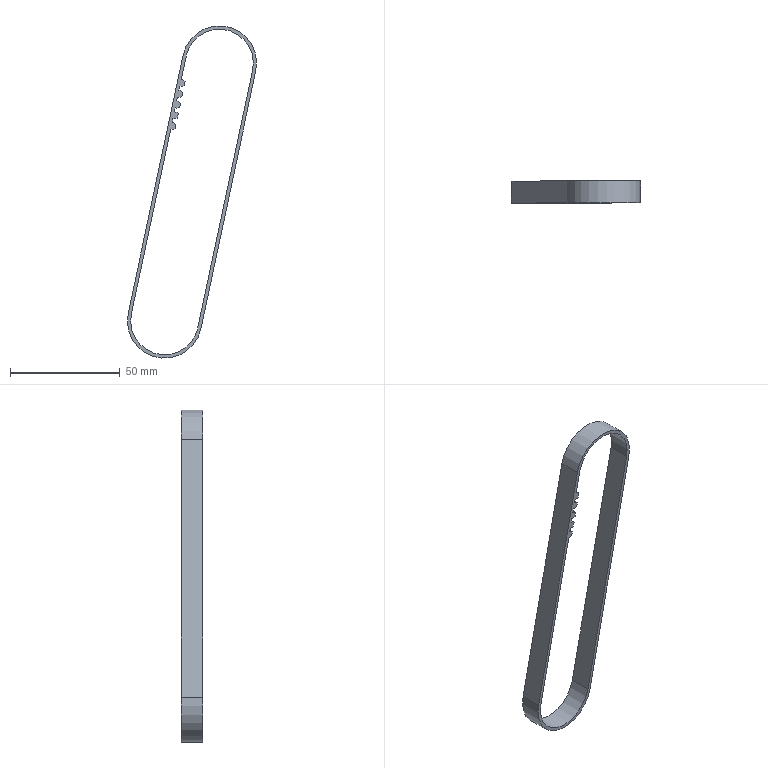Part | STEP file | ROTATION MC_NEW VER-0610_583 | 1 solid | 30 faces | box 58.82 x 10 x 151.249 mm | volume 5398 mm3 | plane 16 | cylinder 14 | commonest cylinder face diameters 6.5 x10 30.871 x2 33.871 x2
STEP:
#1=CARTESIAN_POINT('',(-250.868,696.008,-98.41));
#2=VERTEX_POINT('',#1);
#3=CARTESIAN_POINT('',(-249.129,696.008,-99.414));
#4=VERTEX_POINT('',#3);
#5=CARTESIAN_POINT('',(-251.544,696.008,-101.589));
#6=DIRECTION('',(0.,1.,0.));
#7=DIRECTION('',(-0.2079,0.,-0.9781));
#8=AXIS2_PLACEMENT_3D('',#5,#6,#7);
#9=CIRCLE('',#8,3.25);
#10=EDGE_CURVE('',#2,#4,#9,.T.);
#11=ORIENTED_EDGE('',*,*,#10,.T.);
#12=CARTESIAN_POINT('',(-249.129,706.008,-99.414));
#13=VERTEX_POINT('',#12);
#14=CARTESIAN_POINT('',(-249.129,706.008,-99.414));
#15=DIRECTION('',(0.,-1.,0.));
#16=VECTOR('',#15,10.);
#17=LINE('',#14,#16);
#18=EDGE_CURVE('',#13,#4,#17,.T.);
#19=ORIENTED_EDGE('',*,*,#18,.F.);
#20=CARTESIAN_POINT('',(-250.868,706.008,-98.41));
#21=VERTEX_POINT('',#20);
#22=CARTESIAN_POINT('',(-251.544,706.008,-101.589));
#23=DIRECTION('',(0.,1.,0.));
#24=DIRECTION('',(-0.2079,0.,-0.9781));
#25=AXIS2_PLACEMENT_3D('',#22,#23,#24);
#26=CIRCLE('',#25,3.25);
#27=EDGE_CURVE('',#21,#13,#26,.T.);
#28=ORIENTED_EDGE('',*,*,#27,.F.);
#29=CARTESIAN_POINT('',(-250.868,706.008,-98.41));
#30=DIRECTION('',(0.,-1.,0.));
#31=VECTOR('',#30,10.);
#32=LINE('',#29,#31);
#33=EDGE_CURVE('',#21,#2,#32,.T.);
#34=ORIENTED_EDGE('',*,*,#33,.T.);
#35=EDGE_LOOP('',(#11,#19,#28,#34));
#36=FACE_OUTER_BOUND('',#35,.T.);
#37=CARTESIAN_POINT('',(-251.544,706.008,-101.589));
#38=DIRECTION('',(0.,1.,0.));
#39=DIRECTION('',(-0.2079,0.,-0.9781));
#40=AXIS2_PLACEMENT_3D('',#37,#38,#39);
#41=CYLINDRICAL_SURFACE('',#40,3.25);
#42=ADVANCED_FACE('',(#36),#41,.T.);
#43=CARTESIAN_POINT('',(-249.547,696.008,-101.379));
#44=VERTEX_POINT('',#43);
#45=CARTESIAN_POINT('',(-249.129,696.008,-99.414));
#46=DIRECTION('',(-0.2079,0.,-0.9781));
#47=VECTOR('',#46,2.009);
#48=LINE('',#45,#47);
#49=EDGE_CURVE('',#4,#44,#48,.T.);
#50=ORIENTED_EDGE('',*,*,#49,.T.);
#51=CARTESIAN_POINT('',(-249.547,706.008,-101.379));
#52=VERTEX_POINT('',#51);
#53=CARTESIAN_POINT('',(-249.547,706.008,-101.379));
#54=DIRECTION('',(0.,-1.,0.));
#55=VECTOR('',#54,10.);
#56=LINE('',#53,#55);
#57=EDGE_CURVE('',#52,#44,#56,.T.);
#58=ORIENTED_EDGE('',*,*,#57,.F.);
#59=CARTESIAN_POINT('',(-249.129,706.008,-99.414));
#60=DIRECTION('',(-0.2079,0.,-0.9781));
#61=VECTOR('',#60,2.009);
#62=LINE('',#59,#61);
#63=EDGE_CURVE('',#13,#52,#62,.T.);
#64=ORIENTED_EDGE('',*,*,#63,.F.);
#65=ORIENTED_EDGE('',*,*,#18,.T.);
#66=EDGE_LOOP('',(#50,#58,#64,#65));
#67=FACE_OUTER_BOUND('',#66,.T.);
#68=CARTESIAN_POINT('',(-249.129,706.008,-99.414));
#69=DIRECTION('',(-0.9781,0.,0.2079));
#70=DIRECTION('',(0.2079,0.,0.9781));
#71=AXIS2_PLACEMENT_3D('',#68,#69,#70);
#72=PLANE('',#71);
#73=ADVANCED_FACE('',(#67),#72,.F.);
#74=CARTESIAN_POINT('',(-251.544,696.008,-101.589));
#75=VERTEX_POINT('',#74);
#76=CARTESIAN_POINT('',(-250.868,696.008,-98.41));
#77=DIRECTION('',(0.,1.,0.));
#78=DIRECTION('',(-0.2079,0.,-0.9781));
#79=AXIS2_PLACEMENT_3D('',#76,#77,#78);
#80=CIRCLE('',#79,3.25);
#81=EDGE_CURVE('',#44,#75,#80,.T.);
#82=ORIENTED_EDGE('',*,*,#81,.T.);
#83=CARTESIAN_POINT('',(-251.544,706.008,-101.589));
#84=VERTEX_POINT('',#83);
#85=CARTESIAN_POINT('',(-251.544,706.008,-101.589));
#86=DIRECTION('',(0.,-1.,0.));
#87=VECTOR('',#86,10.);
#88=LINE('',#85,#87);
#89=EDGE_CURVE('',#84,#75,#88,.T.);
#90=ORIENTED_EDGE('',*,*,#89,.F.);
#91=CARTESIAN_POINT('',(-250.868,706.008,-98.41));
#92=DIRECTION('',(0.,1.,0.));
#93=DIRECTION('',(-0.2079,0.,-0.9781));
#94=AXIS2_PLACEMENT_3D('',#91,#92,#93);
#95=CIRCLE('',#94,3.25);
#96=EDGE_CURVE('',#52,#84,#95,.T.);
#97=ORIENTED_EDGE('',*,*,#96,.F.);
#98=ORIENTED_EDGE('',*,*,#57,.T.);
#99=EDGE_LOOP('',(#82,#90,#97,#98));
#100=FACE_OUTER_BOUND('',#99,.T.);
#101=CARTESIAN_POINT('',(-250.868,706.008,-98.41));
#102=DIRECTION('',(0.,1.,0.));
#103=DIRECTION('',(-0.2079,0.,-0.9781));
#104=AXIS2_PLACEMENT_3D('',#101,#102,#103);
#105=CYLINDRICAL_SURFACE('',#104,3.25);
#106=ADVANCED_FACE('',(#100),#105,.T.);
#107=CARTESIAN_POINT('',(-251.908,696.008,-103.301));
#108=VERTEX_POINT('',#107);
#109=CARTESIAN_POINT('',(-251.544,696.008,-101.589));
#110=DIRECTION('',(-0.2079,0.,-0.9781));
#111=VECTOR('',#110,1.75);
#112=LINE('',#109,#111);
#113=EDGE_CURVE('',#75,#108,#112,.T.);
#114=ORIENTED_EDGE('',*,*,#113,.T.);
#115=CARTESIAN_POINT('',(-251.908,706.008,-103.301));
#116=VERTEX_POINT('',#115);
#117=CARTESIAN_POINT('',(-251.908,706.008,-103.301));
#118=DIRECTION('',(0.,-1.,0.));
#119=VECTOR('',#118,10.);
#120=LINE('',#117,#119);
#121=EDGE_CURVE('',#116,#108,#120,.T.);
#122=ORIENTED_EDGE('',*,*,#121,.F.);
#123=CARTESIAN_POINT('',(-251.544,706.008,-101.589));
#124=DIRECTION('',(-0.2079,0.,-0.9781));
#125=VECTOR('',#124,1.75);
#126=LINE('',#123,#125);
#127=EDGE_CURVE('',#84,#116,#126,.T.);
#128=ORIENTED_EDGE('',*,*,#127,.F.);
#129=ORIENTED_EDGE('',*,*,#89,.T.);
#130=EDGE_LOOP('',(#114,#122,#128,#129));
#131=FACE_OUTER_BOUND('',#130,.T.);
#132=CARTESIAN_POINT('',(-251.544,706.008,-101.589));
#133=DIRECTION('',(-0.9781,0.,0.2079));
#134=DIRECTION('',(0.2079,0.,0.9781));
#135=AXIS2_PLACEMENT_3D('',#132,#133,#134);
#136=PLANE('',#135);
#137=ADVANCED_FACE('',(#131),#136,.F.);
#138=CARTESIAN_POINT('',(-250.168,696.008,-104.305));
#139=VERTEX_POINT('',#138);
#140=CARTESIAN_POINT('',(-252.583,696.008,-106.48));
#141=DIRECTION('',(0.,1.,0.));
#142=DIRECTION('',(-0.2079,0.,-0.9781));
#143=AXIS2_PLACEMENT_3D('',#140,#141,#142);
#144=CIRCLE('',#143,3.25);
#145=EDGE_CURVE('',#108,#139,#144,.T.);
#146=ORIENTED_EDGE('',*,*,#145,.T.);
#147=CARTESIAN_POINT('',(-250.168,706.008,-104.305));
#148=VERTEX_POINT('',#147);
#149=CARTESIAN_POINT('',(-250.168,706.008,-104.305));
#150=DIRECTION('',(0.,-1.,0.));
#151=VECTOR('',#150,10.);
#152=LINE('',#149,#151);
#153=EDGE_CURVE('',#148,#139,#152,.T.);
#154=ORIENTED_EDGE('',*,*,#153,.F.);
#155=CARTESIAN_POINT('',(-252.583,706.008,-106.48));
#156=DIRECTION('',(0.,1.,0.));
#157=DIRECTION('',(-0.2079,0.,-0.9781));
#158=AXIS2_PLACEMENT_3D('',#155,#156,#157);
#159=CIRCLE('',#158,3.25);
#160=EDGE_CURVE('',#116,#148,#159,.T.);
#161=ORIENTED_EDGE('',*,*,#160,.F.);
#162=ORIENTED_EDGE('',*,*,#121,.T.);
#163=EDGE_LOOP('',(#146,#154,#161,#162));
#164=FACE_OUTER_BOUND('',#163,.T.);
#165=CARTESIAN_POINT('',(-252.583,706.008,-106.48));
#166=DIRECTION('',(0.,1.,0.));
#167=DIRECTION('',(-0.2079,0.,-0.9781));
#168=AXIS2_PLACEMENT_3D('',#165,#166,#167);
#169=CYLINDRICAL_SURFACE('',#168,3.25);
#170=ADVANCED_FACE('',(#164),#169,.T.);
#171=CARTESIAN_POINT('',(-250.586,696.008,-106.27));
#172=VERTEX_POINT('',#171);
#173=CARTESIAN_POINT('',(-250.168,696.008,-104.305));
#174=DIRECTION('',(-0.2079,0.,-0.9781));
#175=VECTOR('',#174,2.009);
#176=LINE('',#173,#175);
#177=EDGE_CURVE('',#139,#172,#176,.T.);
#178=ORIENTED_EDGE('',*,*,#177,.T.);
#179=CARTESIAN_POINT('',(-250.586,706.008,-106.27));
#180=VERTEX_POINT('',#179);
#181=CARTESIAN_POINT('',(-250.586,706.008,-106.27));
#182=DIRECTION('',(0.,-1.,0.));
#183=VECTOR('',#182,10.);
#184=LINE('',#181,#183);
#185=EDGE_CURVE('',#180,#172,#184,.T.);
#186=ORIENTED_EDGE('',*,*,#185,.F.);
#187=CARTESIAN_POINT('',(-250.168,706.008,-104.305));
#188=DIRECTION('',(-0.2079,0.,-0.9781));
#189=VECTOR('',#188,2.009);
#190=LINE('',#187,#189);
#191=EDGE_CURVE('',#148,#180,#190,.T.);
#192=ORIENTED_EDGE('',*,*,#191,.F.);
#193=ORIENTED_EDGE('',*,*,#153,.T.);
#194=EDGE_LOOP('',(#178,#186,#192,#193));
#195=FACE_OUTER_BOUND('',#194,.T.);
#196=CARTESIAN_POINT('',(-250.168,706.008,-104.305));
#197=DIRECTION('',(-0.9781,0.,0.2079));
#198=DIRECTION('',(0.2079,0.,0.9781));
#199=AXIS2_PLACEMENT_3D('',#196,#197,#198);
#200=PLANE('',#199);
#201=ADVANCED_FACE('',(#195),#200,.F.);
#202=CARTESIAN_POINT('',(-252.583,696.008,-106.48));
#203=VERTEX_POINT('',#202);
#204=CARTESIAN_POINT('',(-251.908,696.008,-103.301));
#205=DIRECTION('',(0.,1.,0.));
#206=DIRECTION('',(-0.2079,0.,-0.9781));
#207=AXIS2_PLACEMENT_3D('',#204,#205,#206);
#208=CIRCLE('',#207,3.25);
#209=EDGE_CURVE('',#172,#203,#208,.T.);
#210=ORIENTED_EDGE('',*,*,#209,.T.);
#211=CARTESIAN_POINT('',(-252.583,706.008,-106.48));
#212=VERTEX_POINT('',#211);
#213=CARTESIAN_POINT('',(-252.583,706.008,-106.48));
#214=DIRECTION('',(0.,-1.,0.));
#215=VECTOR('',#214,10.);
#216=LINE('',#213,#215);
#217=EDGE_CURVE('',#212,#203,#216,.T.);
#218=ORIENTED_EDGE('',*,*,#217,.F.);
#219=CARTESIAN_POINT('',(-251.908,706.008,-103.301));
#220=DIRECTION('',(0.,1.,0.));
#221=DIRECTION('',(-0.2079,0.,-0.9781));
#222=AXIS2_PLACEMENT_3D('',#219,#220,#221);
#223=CIRCLE('',#222,3.25);
#224=EDGE_CURVE('',#180,#212,#223,.T.);
#225=ORIENTED_EDGE('',*,*,#224,.F.);
#226=ORIENTED_EDGE('',*,*,#185,.T.);
#227=EDGE_LOOP('',(#210,#218,#225,#226));
#228=FACE_OUTER_BOUND('',#227,.T.);
#229=CARTESIAN_POINT('',(-251.908,706.008,-103.301));
#230=DIRECTION('',(0.,1.,0.));
#231=DIRECTION('',(-0.2079,0.,-0.9781));
#232=AXIS2_PLACEMENT_3D('',#229,#230,#231);
#233=CYLINDRICAL_SURFACE('',#232,3.25);
#234=ADVANCED_FACE('',(#228),#233,.T.);
#235=CARTESIAN_POINT('',(-252.947,696.008,-108.192));
#236=VERTEX_POINT('',#235);
#237=CARTESIAN_POINT('',(-252.583,696.008,-106.48));
#238=DIRECTION('',(-0.2079,0.,-0.9781));
#239=VECTOR('',#238,1.75);
#240=LINE('',#237,#239);
#241=EDGE_CURVE('',#203,#236,#240,.T.);
#242=ORIENTED_EDGE('',*,*,#241,.T.);
#243=CARTESIAN_POINT('',(-252.947,706.008,-108.192));
#244=VERTEX_POINT('',#243);
#245=CARTESIAN_POINT('',(-252.947,706.008,-108.192));
#246=DIRECTION('',(0.,-1.,0.));
#247=VECTOR('',#246,10.);
#248=LINE('',#245,#247);
#249=EDGE_CURVE('',#244,#236,#248,.T.);
#250=ORIENTED_EDGE('',*,*,#249,.F.);
#251=CARTESIAN_POINT('',(-252.583,706.008,-106.48));
#252=DIRECTION('',(-0.2079,0.,-0.9781));
#253=VECTOR('',#252,1.75);
#254=LINE('',#251,#253);
#255=EDGE_CURVE('',#212,#244,#254,.T.);
#256=ORIENTED_EDGE('',*,*,#255,.F.);
#257=ORIENTED_EDGE('',*,*,#217,.T.);
#258=EDGE_LOOP('',(#242,#250,#256,#257));
#259=FACE_OUTER_BOUND('',#258,.T.);
#260=CARTESIAN_POINT('',(-252.583,706.008,-106.48));
#261=DIRECTION('',(-0.9781,0.,0.2079));
#262=DIRECTION('',(0.2079,0.,0.9781));
#263=AXIS2_PLACEMENT_3D('',#260,#261,#262);
#264=PLANE('',#263);
#265=ADVANCED_FACE('',(#259),#264,.F.);
#266=CARTESIAN_POINT('',(-251.208,696.008,-109.196));
#267=VERTEX_POINT('',#266);
#268=CARTESIAN_POINT('',(-253.623,696.008,-111.371));
#269=DIRECTION('',(0.,1.,0.));
#270=DIRECTION('',(-0.2079,0.,-0.9781));
#271=AXIS2_PLACEMENT_3D('',#268,#269,#270);
#272=CIRCLE('',#271,3.25);
#273=EDGE_CURVE('',#236,#267,#272,.T.);
#274=ORIENTED_EDGE('',*,*,#273,.T.);
#275=CARTESIAN_POINT('',(-251.208,706.008,-109.196));
#276=VERTEX_POINT('',#275);
#277=CARTESIAN_POINT('',(-251.208,706.008,-109.196));
#278=DIRECTION('',(0.,-1.,0.));
#279=VECTOR('',#278,10.);
#280=LINE('',#277,#279);
#281=EDGE_CURVE('',#276,#267,#280,.T.);
#282=ORIENTED_EDGE('',*,*,#281,.F.);
#283=CARTESIAN_POINT('',(-253.623,706.008,-111.371));
#284=DIRECTION('',(0.,1.,0.));
#285=DIRECTION('',(-0.2079,0.,-0.9781));
#286=AXIS2_PLACEMENT_3D('',#283,#284,#285);
#287=CIRCLE('',#286,3.25);
#288=EDGE_CURVE('',#244,#276,#287,.T.);
#289=ORIENTED_EDGE('',*,*,#288,.F.);
#290=ORIENTED_EDGE('',*,*,#249,.T.);
#291=EDGE_LOOP('',(#274,#282,#289,#290));
#292=FACE_OUTER_BOUND('',#291,.T.);
#293=CARTESIAN_POINT('',(-253.623,706.008,-111.371));
#294=DIRECTION('',(0.,1.,0.));
#295=DIRECTION('',(-0.2079,0.,-0.9781));
#296=AXIS2_PLACEMENT_3D('',#293,#294,#295);
#297=CYLINDRICAL_SURFACE('',#296,3.25);
#298=ADVANCED_FACE('',(#292),#297,.T.);
#299=CARTESIAN_POINT('',(-251.626,696.008,-111.161));
#300=VERTEX_POINT('',#299);
#301=CARTESIAN_POINT('',(-251.208,696.008,-109.196));
#302=DIRECTION('',(-0.2079,0.,-0.9781));
#303=VECTOR('',#302,2.009);
#304=LINE('',#301,#303);
#305=EDGE_CURVE('',#267,#300,#304,.T.);
#306=ORIENTED_EDGE('',*,*,#305,.T.);
#307=CARTESIAN_POINT('',(-251.626,706.008,-111.161));
#308=VERTEX_POINT('',#307);
#309=CARTESIAN_POINT('',(-251.626,706.008,-111.161));
#310=DIRECTION('',(0.,-1.,0.));
#311=VECTOR('',#310,10.);
#312=LINE('',#309,#311);
#313=EDGE_CURVE('',#308,#300,#312,.T.);
#314=ORIENTED_EDGE('',*,*,#313,.F.);
#315=CARTESIAN_POINT('',(-251.208,706.008,-109.196));
#316=DIRECTION('',(-0.2079,0.,-0.9781));
#317=VECTOR('',#316,2.009);
#318=LINE('',#315,#317);
#319=EDGE_CURVE('',#276,#308,#318,.T.);
#320=ORIENTED_EDGE('',*,*,#319,.F.);
#321=ORIENTED_EDGE('',*,*,#281,.T.);
#322=EDGE_LOOP('',(#306,#314,#320,#321));
#323=FACE_OUTER_BOUND('',#322,.T.);
#324=CARTESIAN_POINT('',(-251.208,706.008,-109.196));
#325=DIRECTION('',(-0.9781,0.,0.2079));
#326=DIRECTION('',(0.2079,0.,0.9781));
#327=AXIS2_PLACEMENT_3D('',#324,#325,#326);
#328=PLANE('',#327);
#329=ADVANCED_FACE('',(#323),#328,.F.);
#330=CARTESIAN_POINT('',(-252.665,696.008,-116.052));
#331=VERTEX_POINT('',#330);
#332=CARTESIAN_POINT('',(-254.662,696.008,-116.261));
#333=VERTEX_POINT('',#332);
#334=CARTESIAN_POINT('',(-253.987,696.008,-113.082));
#335=DIRECTION('',(0.,1.,0.));
#336=DIRECTION('',(-0.2079,0.,-0.9781));
#337=AXIS2_PLACEMENT_3D('',#334,#335,#336);
#338=CIRCLE('',#337,3.25);
#339=EDGE_CURVE('',#331,#333,#338,.T.);
#340=ORIENTED_EDGE('',*,*,#339,.T.);
#341=CARTESIAN_POINT('',(-254.662,706.008,-116.261));
#342=VERTEX_POINT('',#341);
#343=CARTESIAN_POINT('',(-254.662,706.008,-116.261));
#344=DIRECTION('',(0.,-1.,0.));
#345=VECTOR('',#344,10.);
#346=LINE('',#343,#345);
#347=EDGE_CURVE('',#342,#333,#346,.T.);
#348=ORIENTED_EDGE('',*,*,#347,.F.);
#349=CARTESIAN_POINT('',(-252.665,706.008,-116.052));
#350=VERTEX_POINT('',#349);
#351=CARTESIAN_POINT('',(-253.987,706.008,-113.082));
#352=DIRECTION('',(0.,1.,0.));
#353=DIRECTION('',(-0.2079,0.,-0.9781));
#354=AXIS2_PLACEMENT_3D('',#351,#352,#353);
#355=CIRCLE('',#354,3.25);
#356=EDGE_CURVE('',#350,#342,#355,.T.);
#357=ORIENTED_EDGE('',*,*,#356,.F.);
#358=CARTESIAN_POINT('',(-252.665,706.008,-116.052));
#359=DIRECTION('',(0.,-1.,0.));
#360=VECTOR('',#359,10.);
#361=LINE('',#358,#360);
#362=EDGE_CURVE('',#350,#331,#361,.T.);
#363=ORIENTED_EDGE('',*,*,#362,.T.);
#364=EDGE_LOOP('',(#340,#348,#357,#363));
#365=FACE_OUTER_BOUND('',#364,.T.);
#366=CARTESIAN_POINT('',(-253.987,706.008,-113.082));
#367=DIRECTION('',(0.,1.,0.));
#368=DIRECTION('',(-0.2079,0.,-0.9781));
#369=AXIS2_PLACEMENT_3D('',#366,#367,#368);
#370=CYLINDRICAL_SURFACE('',#369,3.25);
#371=ADVANCED_FACE('',(#365),#370,.T.);
#372=CARTESIAN_POINT('',(-240.853,696.008,-206.99));
#373=VERTEX_POINT('',#372);
#374=CARTESIAN_POINT('',(-273.984,696.008,-199.948));
#375=VERTEX_POINT('',#374);
#376=CARTESIAN_POINT('',(-257.419,696.008,-203.469));
#377=DIRECTION('',(0.,1.,0.));
#378=DIRECTION('',(-0.2079,0.,-0.9781));
#379=AXIS2_PLACEMENT_3D('',#376,#377,#378);
#380=CIRCLE('',#379,16.935);
#381=EDGE_CURVE('',#373,#375,#380,.T.);
#382=ORIENTED_EDGE('',*,*,#381,.T.);
#383=CARTESIAN_POINT('',(-273.984,706.008,-199.948));
#384=VERTEX_POINT('',#383);
#385=CARTESIAN_POINT('',(-273.984,706.008,-199.948));
#386=DIRECTION('',(0.,-1.,0.));
#387=VECTOR('',#386,10.);
#388=LINE('',#385,#387);
#389=EDGE_CURVE('',#384,#375,#388,.T.);
#390=ORIENTED_EDGE('',*,*,#389,.F.);
#391=CARTESIAN_POINT('',(-240.853,706.008,-206.99));
#392=VERTEX_POINT('',#391);
#393=CARTESIAN_POINT('',(-257.419,706.008,-203.469));
#394=DIRECTION('',(0.,1.,0.));
#395=DIRECTION('',(-0.2079,0.,-0.9781));
#396=AXIS2_PLACEMENT_3D('',#393,#394,#395);
#397=CIRCLE('',#396,16.935);
#398=EDGE_CURVE('',#392,#384,#397,.T.);
#399=ORIENTED_EDGE('',*,*,#398,.F.);
#400=CARTESIAN_POINT('',(-240.853,706.008,-206.99));
#401=DIRECTION('',(0.,-1.,0.));
#402=VECTOR('',#401,10.);
#403=LINE('',#400,#402);
#404=EDGE_CURVE('',#392,#373,#403,.T.);
#405=ORIENTED_EDGE('',*,*,#404,.T.);
#406=EDGE_LOOP('',(#382,#390,#399,#405));
#407=FACE_OUTER_BOUND('',#406,.T.);
#408=CARTESIAN_POINT('',(-257.419,706.008,-203.469));
#409=DIRECTION('',(0.,1.,0.));
#410=DIRECTION('',(-0.2079,0.,-0.9781));
#411=AXIS2_PLACEMENT_3D('',#408,#409,#410);
#412=CYLINDRICAL_SURFACE('',#411,16.935);
#413=ADVANCED_FACE('',(#407),#412,.T.);
#414=CARTESIAN_POINT('',(-247.567,696.008,-82.882));
#415=VERTEX_POINT('',#414);
#416=CARTESIAN_POINT('',(-217.371,696.008,-89.301));
#417=VERTEX_POINT('',#416);
#418=CARTESIAN_POINT('',(-232.469,696.008,-86.091));
#419=DIRECTION('',(0.,1.,0.));
#420=DIRECTION('',(-0.2079,0.,-0.9781));
#421=AXIS2_PLACEMENT_3D('',#418,#419,#420);
#422=CIRCLE('',#421,15.435);
#423=EDGE_CURVE('',#415,#417,#422,.T.);
#424=ORIENTED_EDGE('',*,*,#423,.F.);
#425=CARTESIAN_POINT('',(-247.567,706.008,-82.882));
#426=VERTEX_POINT('',#425);
#427=CARTESIAN_POINT('',(-247.567,706.008,-82.882));
#428=DIRECTION('',(0.,-1.,0.));
#429=VECTOR('',#428,10.);
#430=LINE('',#427,#429);
#431=EDGE_CURVE('',#426,#415,#430,.T.);
#432=ORIENTED_EDGE('',*,*,#431,.F.);
#433=CARTESIAN_POINT('',(-217.371,706.008,-89.301));
#434=VERTEX_POINT('',#433);
#435=CARTESIAN_POINT('',(-232.469,706.008,-86.091));
#436=DIRECTION('',(0.,1.,0.));
#437=DIRECTION('',(-0.2079,0.,-0.9781));
#438=AXIS2_PLACEMENT_3D('',#435,#436,#437);
#439=CIRCLE('',#438,15.435);
#440=EDGE_CURVE('',#426,#434,#439,.T.);
#441=ORIENTED_EDGE('',*,*,#440,.T.);
#442=CARTESIAN_POINT('',(-217.371,706.008,-89.301));
#443=DIRECTION('',(0.,-1.,0.));
#444=VECTOR('',#443,10.);
#445=LINE('',#442,#444);
#446=EDGE_CURVE('',#434,#417,#445,.T.);
#447=ORIENTED_EDGE('',*,*,#446,.T.);
#448=EDGE_LOOP('',(#424,#432,#441,#447));
#449=FACE_OUTER_BOUND('',#448,.T.);
#450=CARTESIAN_POINT('',(-232.469,706.008,-86.091));
#451=DIRECTION('',(0.,1.,0.));
#452=DIRECTION('',(0.2079,0.,0.9781));
#453=AXIS2_PLACEMENT_3D('',#450,#451,#452);
#454=CYLINDRICAL_SURFACE('',#453,15.435);
#455=ADVANCED_FACE('',(#449),#454,.F.);
#456=CARTESIAN_POINT('',(-242.321,696.008,-206.678));
#457=VERTEX_POINT('',#456);
#458=CARTESIAN_POINT('',(-217.371,696.008,-89.301));
#459=DIRECTION('',(-0.2079,0.,-0.9781));
#460=VECTOR('',#459,120.);
#461=LINE('',#458,#460);
#462=EDGE_CURVE('',#417,#457,#461,.T.);
#463=ORIENTED_EDGE('',*,*,#462,.F.);
#464=ORIENTED_EDGE('',*,*,#446,.F.);
#465=CARTESIAN_POINT('',(-242.321,706.008,-206.678));
#466=VERTEX_POINT('',#465);
#467=CARTESIAN_POINT('',(-217.371,706.008,-89.301));
#468=DIRECTION('',(-0.2079,0.,-0.9781));
#469=VECTOR('',#468,120.);
#470=LINE('',#467,#469);
#471=EDGE_CURVE('',#434,#466,#470,.T.);
#472=ORIENTED_EDGE('',*,*,#471,.T.);
#473=CARTESIAN_POINT('',(-242.321,706.008,-206.678));
#474=DIRECTION('',(0.,-1.,0.));
#475=VECTOR('',#474,10.);
#476=LINE('',#473,#475);
#477=EDGE_CURVE('',#466,#457,#476,.T.);
#478=ORIENTED_EDGE('',*,*,#477,.T.);
#479=EDGE_LOOP('',(#463,#464,#472,#478));
#480=FACE_OUTER_BOUND('',#479,.T.);
#481=CARTESIAN_POINT('',(-217.371,706.008,-89.301));
#482=DIRECTION('',(-0.9781,0.,0.2079));
#483=DIRECTION('',(0.2079,0.,0.9781));
#484=AXIS2_PLACEMENT_3D('',#481,#482,#483);
#485=PLANE('',#484);
#486=ADVANCED_FACE('',(#480),#485,.T.);
#487=CARTESIAN_POINT('',(-215.904,696.008,-89.612));
#488=VERTEX_POINT('',#487);
#489=CARTESIAN_POINT('',(-215.904,696.008,-89.612));
#490=DIRECTION('',(-0.2079,0.,-0.9781));
#491=VECTOR('',#490,120.);
#492=LINE('',#489,#491);
#493=EDGE_CURVE('',#488,#373,#492,.T.);
#494=ORIENTED_EDGE('',*,*,#493,.T.);
#495=ORIENTED_EDGE('',*,*,#404,.F.);
#496=CARTESIAN_POINT('',(-215.904,706.008,-89.612));
#497=VERTEX_POINT('',#496);
#498=CARTESIAN_POINT('',(-215.904,706.008,-89.612));
#499=DIRECTION('',(-0.2079,0.,-0.9781));
#500=VECTOR('',#499,120.);
#501=LINE('',#498,#500);
#502=EDGE_CURVE('',#497,#392,#501,.T.);
#503=ORIENTED_EDGE('',*,*,#502,.F.);
#504=CARTESIAN_POINT('',(-215.904,706.008,-89.612));
#505=DIRECTION('',(0.,-1.,0.));
#506=VECTOR('',#505,10.);
#507=LINE('',#504,#506);
#508=EDGE_CURVE('',#497,#488,#507,.T.);
#509=ORIENTED_EDGE('',*,*,#508,.T.);
#510=EDGE_LOOP('',(#494,#495,#503,#509));
#511=FACE_OUTER_BOUND('',#510,.T.);
#512=CARTESIAN_POINT('',(-215.904,706.008,-89.612));
#513=DIRECTION('',(-0.9781,0.,0.2079));
#514=DIRECTION('',(0.2079,0.,0.9781));
#515=AXIS2_PLACEMENT_3D('',#512,#513,#514);
#516=PLANE('',#515);
#517=ADVANCED_FACE('',(#511),#516,.F.);
#518=CARTESIAN_POINT('',(-249.035,696.008,-82.57));
#519=VERTEX_POINT('',#518);
#520=CARTESIAN_POINT('',(-232.469,696.008,-86.091));
#521=DIRECTION('',(0.,1.,0.));
#522=DIRECTION('',(-0.2079,0.,-0.9781));
#523=AXIS2_PLACEMENT_3D('',#520,#521,#522);
#524=CIRCLE('',#523,16.935);
#525=EDGE_CURVE('',#519,#488,#524,.T.);
#526=ORIENTED_EDGE('',*,*,#525,.T.);
#527=ORIENTED_EDGE('',*,*,#508,.F.);
#528=CARTESIAN_POINT('',(-249.035,706.008,-82.57));
#529=VERTEX_POINT('',#528);
#530=CARTESIAN_POINT('',(-232.469,706.008,-86.091));
#531=DIRECTION('',(0.,1.,0.));
#532=DIRECTION('',(-0.2079,0.,-0.9781));
#533=AXIS2_PLACEMENT_3D('',#530,#531,#532);
#534=CIRCLE('',#533,16.935);
#535=EDGE_CURVE('',#529,#497,#534,.T.);
#536=ORIENTED_EDGE('',*,*,#535,.F.);
#537=CARTESIAN_POINT('',(-249.035,706.008,-82.57));
#538=DIRECTION('',(0.,-1.,0.));
#539=VECTOR('',#538,10.);
#540=LINE('',#537,#539);
#541=EDGE_CURVE('',#529,#519,#540,.T.);
#542=ORIENTED_EDGE('',*,*,#541,.T.);
#543=EDGE_LOOP('',(#526,#527,#536,#542));
#544=FACE_OUTER_BOUND('',#543,.T.);
#545=CARTESIAN_POINT('',(-232.469,706.008,-86.091));
#546=DIRECTION('',(0.,1.,0.));
#547=DIRECTION('',(0.2079,0.,0.9781));
#548=AXIS2_PLACEMENT_3D('',#545,#546,#547);
#549=CYLINDRICAL_SURFACE('',#548,16.935);
#550=ADVANCED_FACE('',(#544),#549,.T.);
#551=CARTESIAN_POINT('',(-249.829,696.008,-93.519));
#552=VERTEX_POINT('',#551);
#553=CARTESIAN_POINT('',(-247.567,696.008,-82.882));
#554=DIRECTION('',(-0.2079,0.,-0.9781));
#555=VECTOR('',#554,10.875);
#556=LINE('',#553,#555);
#557=EDGE_CURVE('',#415,#552,#556,.T.);
#558=ORIENTED_EDGE('',*,*,#557,.T.);
#559=CARTESIAN_POINT('',(-249.829,706.008,-93.519));
#560=VERTEX_POINT('',#559);
#561=CARTESIAN_POINT('',(-249.829,706.008,-93.519));
#562=DIRECTION('',(0.,-1.,0.));
#563=VECTOR('',#562,10.);
#564=LINE('',#561,#563);
#565=EDGE_CURVE('',#560,#552,#564,.T.);
#566=ORIENTED_EDGE('',*,*,#565,.F.);
#567=CARTESIAN_POINT('',(-247.567,706.008,-82.882));
#568=DIRECTION('',(-0.2079,0.,-0.9781));
#569=VECTOR('',#568,10.875);
#570=LINE('',#567,#569);
#571=EDGE_CURVE('',#426,#560,#570,.T.);
#572=ORIENTED_EDGE('',*,*,#571,.F.);
#573=ORIENTED_EDGE('',*,*,#431,.T.);
#574=EDGE_LOOP('',(#558,#566,#572,#573));
#575=FACE_OUTER_BOUND('',#574,.T.);
#576=CARTESIAN_POINT('',(-249.647,706.008,-92.664));
#577=DIRECTION('',(-0.9781,0.,0.2079));
#578=DIRECTION('',(0.2079,0.,0.9781));
#579=AXIS2_PLACEMENT_3D('',#576,#577,#578);
#580=PLANE('',#579);
#581=ADVANCED_FACE('',(#575),#580,.F.);
#582=CARTESIAN_POINT('',(-248.089,696.008,-94.523));
#583=VERTEX_POINT('',#582);
#584=CARTESIAN_POINT('',(-250.504,696.008,-96.698));
#585=DIRECTION('',(0.,1.,0.));
#586=DIRECTION('',(-0.2079,0.,-0.9781));
#587=AXIS2_PLACEMENT_3D('',#584,#585,#586);
#588=CIRCLE('',#587,3.25);
#589=EDGE_CURVE('',#552,#583,#588,.T.);
#590=ORIENTED_EDGE('',*,*,#589,.T.);
#591=CARTESIAN_POINT('',(-248.089,706.008,-94.523));
#592=VERTEX_POINT('',#591);
#593=CARTESIAN_POINT('',(-248.089,706.008,-94.523));
#594=DIRECTION('',(0.,-1.,0.));
#595=VECTOR('',#594,10.);
#596=LINE('',#593,#595);
#597=EDGE_CURVE('',#592,#583,#596,.T.);
#598=ORIENTED_EDGE('',*,*,#597,.F.);
#599=CARTESIAN_POINT('',(-250.504,706.008,-96.698));
#600=DIRECTION('',(0.,1.,0.));
#601=DIRECTION('',(-0.2079,0.,-0.9781));
#602=AXIS2_PLACEMENT_3D('',#599,#600,#601);
#603=CIRCLE('',#602,3.25);
#604=EDGE_CURVE('',#560,#592,#603,.T.);
#605=ORIENTED_EDGE('',*,*,#604,.F.);
#606=ORIENTED_EDGE('',*,*,#565,.T.);
#607=EDGE_LOOP('',(#590,#598,#605,#606));
#608=FACE_OUTER_BOUND('',#607,.T.);
#609=CARTESIAN_POINT('',(-250.504,706.008,-96.698));
#610=DIRECTION('',(0.,1.,0.));
#611=DIRECTION('',(-0.2079,0.,-0.9781));
#612=AXIS2_PLACEMENT_3D('',#609,#610,#611);
#613=CYLINDRICAL_SURFACE('',#612,3.25);
#614=ADVANCED_FACE('',(#608),#613,.T.);
#615=CARTESIAN_POINT('',(-272.517,696.008,-200.26));
#616=VERTEX_POINT('',#615);
#617=CARTESIAN_POINT('',(-257.419,696.008,-203.469));
#618=DIRECTION('',(0.,1.,0.));
#619=DIRECTION('',(-0.2079,0.,-0.9781));
#620=AXIS2_PLACEMENT_3D('',#617,#618,#619);
#621=CIRCLE('',#620,15.435);
#622=EDGE_CURVE('',#457,#616,#621,.T.);
#623=ORIENTED_EDGE('',*,*,#622,.F.);
#624=ORIENTED_EDGE('',*,*,#477,.F.);
#625=CARTESIAN_POINT('',(-272.517,706.008,-200.26));
#626=VERTEX_POINT('',#625);
#627=CARTESIAN_POINT('',(-257.419,706.008,-203.469));
#628=DIRECTION('',(0.,1.,0.));
#629=DIRECTION('',(-0.2079,0.,-0.9781));
#630=AXIS2_PLACEMENT_3D('',#627,#628,#629);
#631=CIRCLE('',#630,15.435);
#632=EDGE_CURVE('',#466,#626,#631,.T.);
#633=ORIENTED_EDGE('',*,*,#632,.T.);
#634=CARTESIAN_POINT('',(-272.517,706.008,-200.26));
#635=DIRECTION('',(0.,-1.,0.));
#636=VECTOR('',#635,10.);
#637=LINE('',#634,#636);
#638=EDGE_CURVE('',#626,#616,#637,.T.);
#639=ORIENTED_EDGE('',*,*,#638,.T.);
#640=EDGE_LOOP('',(#623,#624,#633,#639));
#641=FACE_OUTER_BOUND('',#640,.T.);
#642=CARTESIAN_POINT('',(-257.419,706.008,-203.469));
#643=DIRECTION('',(0.,1.,0.));
#644=DIRECTION('',(-0.2079,0.,-0.9781));
#645=AXIS2_PLACEMENT_3D('',#642,#643,#644);
#646=CYLINDRICAL_SURFACE('',#645,15.435);
#647=ADVANCED_FACE('',(#641),#646,.F.);
#648=CARTESIAN_POINT('',(-254.662,696.008,-116.261));
#649=DIRECTION('',(-0.2079,0.,-0.9781));
#650=VECTOR('',#649,85.875);
#651=LINE('',#648,#650);
#652=EDGE_CURVE('',#333,#616,#651,.T.);
#653=ORIENTED_EDGE('',*,*,#652,.T.);
#654=ORIENTED_EDGE('',*,*,#638,.F.);
#655=CARTESIAN_POINT('',(-254.662,706.008,-116.261));
#656=DIRECTION('',(-0.2079,0.,-0.9781));
#657=VECTOR('',#656,85.875);
#658=LINE('',#655,#657);
#659=EDGE_CURVE('',#342,#626,#658,.T.);
#660=ORIENTED_EDGE('',*,*,#659,.F.);
#661=ORIENTED_EDGE('',*,*,#347,.T.);
#662=EDGE_LOOP('',(#653,#654,#660,#661));
#663=FACE_OUTER_BOUND('',#662,.T.);
#664=CARTESIAN_POINT('',(-254.662,706.008,-116.261));
#665=DIRECTION('',(-0.9781,0.,0.2079));
#666=DIRECTION('',(0.2079,0.,0.9781));
#667=AXIS2_PLACEMENT_3D('',#664,#665,#666);
#668=PLANE('',#667);
#669=ADVANCED_FACE('',(#663),#668,.F.);
#670=CARTESIAN_POINT('',(-253.623,696.008,-111.371));
#671=VERTEX_POINT('',#670);
#672=CARTESIAN_POINT('',(-253.987,696.008,-113.082));
#673=VERTEX_POINT('',#672);
#674=CARTESIAN_POINT('',(-253.623,696.008,-111.371));
#675=DIRECTION('',(-0.2079,0.,-0.9781));
#676=VECTOR('',#675,1.75);
#677=LINE('',#674,#676);
#678=EDGE_CURVE('',#671,#673,#677,.T.);
#679=ORIENTED_EDGE('',*,*,#678,.T.);
#680=CARTESIAN_POINT('',(-253.987,706.008,-113.082));
#681=VERTEX_POINT('',#680);
#682=CARTESIAN_POINT('',(-253.987,706.008,-113.082));
#683=DIRECTION('',(0.,-1.,0.));
#684=VECTOR('',#683,10.);
#685=LINE('',#682,#684);
#686=EDGE_CURVE('',#681,#673,#685,.T.);
#687=ORIENTED_EDGE('',*,*,#686,.F.);
#688=CARTESIAN_POINT('',(-253.623,706.008,-111.371));
#689=VERTEX_POINT('',#688);
#690=CARTESIAN_POINT('',(-253.623,706.008,-111.371));
#691=DIRECTION('',(-0.2079,0.,-0.9781));
#692=VECTOR('',#691,1.75);
#693=LINE('',#690,#692);
#694=EDGE_CURVE('',#689,#681,#693,.T.);
#695=ORIENTED_EDGE('',*,*,#694,.F.);
#696=CARTESIAN_POINT('',(-253.623,706.008,-111.371));
#697=DIRECTION('',(0.,-1.,0.));
#698=VECTOR('',#697,10.);
#699=LINE('',#696,#698);
#700=EDGE_CURVE('',#689,#671,#699,.T.);
#701=ORIENTED_EDGE('',*,*,#700,.T.);
#702=EDGE_LOOP('',(#679,#687,#695,#701));
#703=FACE_OUTER_BOUND('',#702,.T.);
#704=CARTESIAN_POINT('',(-253.623,706.008,-111.371));
#705=DIRECTION('',(-0.9781,0.,0.2079));
#706=DIRECTION('',(0.2079,0.,0.9781));
#707=AXIS2_PLACEMENT_3D('',#704,#705,#706);
#708=PLANE('',#707);
#709=ADVANCED_FACE('',(#703),#708,.F.);
#710=CARTESIAN_POINT('',(-252.947,696.008,-108.192));
#711=DIRECTION('',(0.,1.,0.));
#712=DIRECTION('',(-0.2079,0.,-0.9781));
#713=AXIS2_PLACEMENT_3D('',#710,#711,#712);
#714=CIRCLE('',#713,3.25);
#715=EDGE_CURVE('',#300,#671,#714,.T.);
#716=ORIENTED_EDGE('',*,*,#715,.T.);
#717=ORIENTED_EDGE('',*,*,#700,.F.);
#718=CARTESIAN_POINT('',(-252.947,706.008,-108.192));
#719=DIRECTION('',(0.,1.,0.));
#720=DIRECTION('',(-0.2079,0.,-0.9781));
#721=AXIS2_PLACEMENT_3D('',#718,#719,#720);
#722=CIRCLE('',#721,3.25);
#723=EDGE_CURVE('',#308,#689,#722,.T.);
#724=ORIENTED_EDGE('',*,*,#723,.F.);
#725=ORIENTED_EDGE('',*,*,#313,.T.);
#726=EDGE_LOOP('',(#716,#717,#724,#725));
#727=FACE_OUTER_BOUND('',#726,.T.);
#728=CARTESIAN_POINT('',(-252.947,706.008,-108.192));
#729=DIRECTION('',(0.,1.,0.));
#730=DIRECTION('',(-0.2079,0.,-0.9781));
#731=AXIS2_PLACEMENT_3D('',#728,#729,#730);
#732=CYLINDRICAL_SURFACE('',#731,3.25);
#733=ADVANCED_FACE('',(#727),#732,.T.);
#734=CARTESIAN_POINT('',(-250.504,696.008,-96.698));
#735=VERTEX_POINT('',#734);
#736=CARTESIAN_POINT('',(-250.504,696.008,-96.698));
#737=DIRECTION('',(-0.2079,0.,-0.9781));
#738=VECTOR('',#737,1.75);
#739=LINE('',#736,#738);
#740=EDGE_CURVE('',#735,#2,#739,.T.);
#741=ORIENTED_EDGE('',*,*,#740,.T.);
#742=ORIENTED_EDGE('',*,*,#33,.F.);
#743=CARTESIAN_POINT('',(-250.504,706.008,-96.698));
#744=VERTEX_POINT('',#743);
#745=CARTESIAN_POINT('',(-250.504,706.008,-96.698));
#746=DIRECTION('',(-0.2079,0.,-0.9781));
#747=VECTOR('',#746,1.75);
#748=LINE('',#745,#747);
#749=EDGE_CURVE('',#744,#21,#748,.T.);
#750=ORIENTED_EDGE('',*,*,#749,.F.);
#751=CARTESIAN_POINT('',(-250.504,706.008,-96.698));
#752=DIRECTION('',(0.,-1.,0.));
#753=VECTOR('',#752,10.);
#754=LINE('',#751,#753);
#755=EDGE_CURVE('',#744,#735,#754,.T.);
#756=ORIENTED_EDGE('',*,*,#755,.T.);
#757=EDGE_LOOP('',(#741,#742,#750,#756));
#758=FACE_OUTER_BOUND('',#757,.T.);
#759=CARTESIAN_POINT('',(-250.504,706.008,-96.698));
#760=DIRECTION('',(-0.9781,0.,0.2079));
#761=DIRECTION('',(0.2079,0.,0.9781));
#762=AXIS2_PLACEMENT_3D('',#759,#760,#761);
#763=PLANE('',#762);
#764=ADVANCED_FACE('',(#758),#763,.F.);
#765=CARTESIAN_POINT('',(-248.507,696.008,-96.489));
#766=VERTEX_POINT('',#765);
#767=CARTESIAN_POINT('',(-249.829,696.008,-93.519));
#768=DIRECTION('',(0.,1.,0.));
#769=DIRECTION('',(-0.2079,0.,-0.9781));
#770=AXIS2_PLACEMENT_3D('',#767,#768,#769);
#771=CIRCLE('',#770,3.25);
#772=EDGE_CURVE('',#766,#735,#771,.T.);
#773=ORIENTED_EDGE('',*,*,#772,.T.);
#774=ORIENTED_EDGE('',*,*,#755,.F.);
#775=CARTESIAN_POINT('',(-248.507,706.008,-96.489));
#776=VERTEX_POINT('',#775);
#777=CARTESIAN_POINT('',(-249.829,706.008,-93.519));
#778=DIRECTION('',(0.,1.,0.));
#779=DIRECTION('',(-0.2079,0.,-0.9781));
#780=AXIS2_PLACEMENT_3D('',#777,#778,#779);
#781=CIRCLE('',#780,3.25);
#782=EDGE_CURVE('',#776,#744,#781,.T.);
#783=ORIENTED_EDGE('',*,*,#782,.F.);
#784=CARTESIAN_POINT('',(-248.507,706.008,-96.489));
#785=DIRECTION('',(0.,-1.,0.));
#786=VECTOR('',#785,10.);
#787=LINE('',#784,#786);
#788=EDGE_CURVE('',#776,#766,#787,.T.);
#789=ORIENTED_EDGE('',*,*,#788,.T.);
#790=EDGE_LOOP('',(#773,#774,#783,#789));
#791=FACE_OUTER_BOUND('',#790,.T.);
#792=CARTESIAN_POINT('',(-249.829,706.008,-93.519));
#793=DIRECTION('',(0.,1.,0.));
#794=DIRECTION('',(-0.2079,0.,-0.9781));
#795=AXIS2_PLACEMENT_3D('',#792,#793,#794);
#796=CYLINDRICAL_SURFACE('',#795,3.25);
#797=ADVANCED_FACE('',(#791),#796,.T.);
#798=ORIENTED_EDGE('',*,*,#525,.F.);
#799=CARTESIAN_POINT('',(-273.984,696.008,-199.948));
#800=DIRECTION('',(0.2079,0.,0.9781));
#801=VECTOR('',#800,120.);
#802=LINE('',#799,#801);
#803=EDGE_CURVE('',#375,#519,#802,.T.);
#804=ORIENTED_EDGE('',*,*,#803,.F.);
#805=ORIENTED_EDGE('',*,*,#381,.F.);
#806=ORIENTED_EDGE('',*,*,#493,.F.);
#807=EDGE_LOOP('',(#798,#804,#805,#806));
#808=FACE_OUTER_BOUND('',#807,.T.);
#809=ORIENTED_EDGE('',*,*,#557,.F.);
#810=ORIENTED_EDGE('',*,*,#423,.T.);
#811=ORIENTED_EDGE('',*,*,#462,.T.);
#812=ORIENTED_EDGE('',*,*,#622,.T.);
#813=ORIENTED_EDGE('',*,*,#652,.F.);
#814=ORIENTED_EDGE('',*,*,#339,.F.);
#815=CARTESIAN_POINT('',(-252.248,696.008,-114.086));
#816=VERTEX_POINT('',#815);
#817=CARTESIAN_POINT('',(-252.248,696.008,-114.086));
#818=DIRECTION('',(-0.2079,0.,-0.9781));
#819=VECTOR('',#818,2.009);
#820=LINE('',#817,#819);
#821=EDGE_CURVE('',#816,#331,#820,.T.);
#822=ORIENTED_EDGE('',*,*,#821,.F.);
#823=CARTESIAN_POINT('',(-254.662,696.008,-116.261));
#824=DIRECTION('',(0.,1.,0.));
#825=DIRECTION('',(-0.2079,0.,-0.9781));
#826=AXIS2_PLACEMENT_3D('',#823,#824,#825);
#827=CIRCLE('',#826,3.25);
#828=EDGE_CURVE('',#673,#816,#827,.T.);
#829=ORIENTED_EDGE('',*,*,#828,.F.);
#830=ORIENTED_EDGE('',*,*,#678,.F.);
#831=ORIENTED_EDGE('',*,*,#715,.F.);
#832=ORIENTED_EDGE('',*,*,#305,.F.);
#833=ORIENTED_EDGE('',*,*,#273,.F.);
#834=ORIENTED_EDGE('',*,*,#241,.F.);
#835=ORIENTED_EDGE('',*,*,#209,.F.);
#836=ORIENTED_EDGE('',*,*,#177,.F.);
#837=ORIENTED_EDGE('',*,*,#145,.F.);
#838=ORIENTED_EDGE('',*,*,#113,.F.);
#839=ORIENTED_EDGE('',*,*,#81,.F.);
#840=ORIENTED_EDGE('',*,*,#49,.F.);
#841=ORIENTED_EDGE('',*,*,#10,.F.);
#842=ORIENTED_EDGE('',*,*,#740,.F.);
#843=ORIENTED_EDGE('',*,*,#772,.F.);
#844=CARTESIAN_POINT('',(-248.089,696.008,-94.523));
#845=DIRECTION('',(-0.2079,0.,-0.9781));
#846=VECTOR('',#845,2.009);
#847=LINE('',#844,#846);
#848=EDGE_CURVE('',#583,#766,#847,.T.);
#849=ORIENTED_EDGE('',*,*,#848,.F.);
#850=ORIENTED_EDGE('',*,*,#589,.F.);
#851=EDGE_LOOP('',(#809,#810,#811,#812,#813,#814,#822,#829,#830,#831,#832,#833,#834,#835,#836,#837,#838,#839,#840,#841,#842,#843,#849,#850));
#852=FACE_BOUND('',#851,.T.);
#853=CARTESIAN_POINT('',(-250.504,696.008,-96.698));
#854=DIRECTION('',(0.,1.,0.));
#855=DIRECTION('',(0.,0.,1.));
#856=AXIS2_PLACEMENT_3D('',#853,#854,#855);
#857=PLANE('',#856);
#858=ADVANCED_FACE('',(#808,#852),#857,.F.);
#859=ORIENTED_EDGE('',*,*,#848,.T.);
#860=ORIENTED_EDGE('',*,*,#788,.F.);
#861=CARTESIAN_POINT('',(-248.089,706.008,-94.523));
#862=DIRECTION('',(-0.2079,0.,-0.9781));
#863=VECTOR('',#862,2.009);
#864=LINE('',#861,#863);
#865=EDGE_CURVE('',#592,#776,#864,.T.);
#866=ORIENTED_EDGE('',*,*,#865,.F.);
#867=ORIENTED_EDGE('',*,*,#597,.T.);
#868=EDGE_LOOP('',(#859,#860,#866,#867));
#869=FACE_OUTER_BOUND('',#868,.T.);
#870=CARTESIAN_POINT('',(-248.089,706.008,-94.523));
#871=DIRECTION('',(-0.9781,0.,0.2079));
#872=DIRECTION('',(0.2079,0.,0.9781));
#873=AXIS2_PLACEMENT_3D('',#870,#871,#872);
#874=PLANE('',#873);
#875=ADVANCED_FACE('',(#869),#874,.F.);
#876=ORIENTED_EDGE('',*,*,#821,.T.);
#877=ORIENTED_EDGE('',*,*,#362,.F.);
#878=CARTESIAN_POINT('',(-252.248,706.008,-114.086));
#879=VERTEX_POINT('',#878);
#880=CARTESIAN_POINT('',(-252.248,706.008,-114.086));
#881=DIRECTION('',(-0.2079,0.,-0.9781));
#882=VECTOR('',#881,2.009);
#883=LINE('',#880,#882);
#884=EDGE_CURVE('',#879,#350,#883,.T.);
#885=ORIENTED_EDGE('',*,*,#884,.F.);
#886=CARTESIAN_POINT('',(-252.248,706.008,-114.086));
#887=DIRECTION('',(0.,-1.,0.));
#888=VECTOR('',#887,10.);
#889=LINE('',#886,#888);
#890=EDGE_CURVE('',#879,#816,#889,.T.);
#891=ORIENTED_EDGE('',*,*,#890,.T.);
#892=EDGE_LOOP('',(#876,#877,#885,#891));
#893=FACE_OUTER_BOUND('',#892,.T.);
#894=CARTESIAN_POINT('',(-252.248,706.008,-114.086));
#895=DIRECTION('',(-0.9781,0.,0.2079));
#896=DIRECTION('',(0.2079,0.,0.9781));
#897=AXIS2_PLACEMENT_3D('',#894,#895,#896);
#898=PLANE('',#897);
#899=ADVANCED_FACE('',(#893),#898,.F.);
#900=ORIENTED_EDGE('',*,*,#828,.T.);
#901=ORIENTED_EDGE('',*,*,#890,.F.);
#902=CARTESIAN_POINT('',(-254.662,706.008,-116.261));
#903=DIRECTION('',(0.,1.,0.));
#904=DIRECTION('',(-0.2079,0.,-0.9781));
#905=AXIS2_PLACEMENT_3D('',#902,#903,#904);
#906=CIRCLE('',#905,3.25);
#907=EDGE_CURVE('',#681,#879,#906,.T.);
#908=ORIENTED_EDGE('',*,*,#907,.F.);
#909=ORIENTED_EDGE('',*,*,#686,.T.);
#910=EDGE_LOOP('',(#900,#901,#908,#909));
#911=FACE_OUTER_BOUND('',#910,.T.);
#912=CARTESIAN_POINT('',(-254.662,706.008,-116.261));
#913=DIRECTION('',(0.,1.,0.));
#914=DIRECTION('',(-0.2079,0.,-0.9781));
#915=AXIS2_PLACEMENT_3D('',#912,#913,#914);
#916=CYLINDRICAL_SURFACE('',#915,3.25);
#917=ADVANCED_FACE('',(#911),#916,.T.);
#918=CARTESIAN_POINT('',(-273.984,706.008,-199.948));
#919=DIRECTION('',(0.2079,0.,0.9781));
#920=VECTOR('',#919,120.);
#921=LINE('',#918,#920);
#922=EDGE_CURVE('',#384,#529,#921,.T.);
#923=ORIENTED_EDGE('',*,*,#922,.T.);
#924=ORIENTED_EDGE('',*,*,#535,.T.);
#925=ORIENTED_EDGE('',*,*,#502,.T.);
#926=ORIENTED_EDGE('',*,*,#398,.T.);
#927=EDGE_LOOP('',(#923,#924,#925,#926));
#928=FACE_OUTER_BOUND('',#927,.T.);
#929=ORIENTED_EDGE('',*,*,#440,.F.);
#930=ORIENTED_EDGE('',*,*,#571,.T.);
#931=ORIENTED_EDGE('',*,*,#604,.T.);
#932=ORIENTED_EDGE('',*,*,#865,.T.);
#933=ORIENTED_EDGE('',*,*,#782,.T.);
#934=ORIENTED_EDGE('',*,*,#749,.T.);
#935=ORIENTED_EDGE('',*,*,#27,.T.);
#936=ORIENTED_EDGE('',*,*,#63,.T.);
#937=ORIENTED_EDGE('',*,*,#96,.T.);
#938=ORIENTED_EDGE('',*,*,#127,.T.);
#939=ORIENTED_EDGE('',*,*,#160,.T.);
#940=ORIENTED_EDGE('',*,*,#191,.T.);
#941=ORIENTED_EDGE('',*,*,#224,.T.);
#942=ORIENTED_EDGE('',*,*,#255,.T.);
#943=ORIENTED_EDGE('',*,*,#288,.T.);
#944=ORIENTED_EDGE('',*,*,#319,.T.);
#945=ORIENTED_EDGE('',*,*,#723,.T.);
#946=ORIENTED_EDGE('',*,*,#694,.T.);
#947=ORIENTED_EDGE('',*,*,#907,.T.);
#948=ORIENTED_EDGE('',*,*,#884,.T.);
#949=ORIENTED_EDGE('',*,*,#356,.T.);
#950=ORIENTED_EDGE('',*,*,#659,.T.);
#951=ORIENTED_EDGE('',*,*,#632,.F.);
#952=ORIENTED_EDGE('',*,*,#471,.F.);
#953=EDGE_LOOP('',(#929,#930,#931,#932,#933,#934,#935,#936,#937,#938,#939,#940,#941,#942,#943,#944,#945,#946,#947,#948,#949,#950,#951,#952));
#954=FACE_BOUND('',#953,.T.);
#955=CARTESIAN_POINT('',(-250.504,706.008,-96.698));
#956=DIRECTION('',(0.,1.,0.));
#957=DIRECTION('',(0.,0.,1.));
#958=AXIS2_PLACEMENT_3D('',#955,#956,#957);
#959=PLANE('',#958);
#960=ADVANCED_FACE('',(#928,#954),#959,.T.);
#961=ORIENTED_EDGE('',*,*,#803,.T.);
#962=ORIENTED_EDGE('',*,*,#541,.F.);
#963=ORIENTED_EDGE('',*,*,#922,.F.);
#964=ORIENTED_EDGE('',*,*,#389,.T.);
#965=EDGE_LOOP('',(#961,#962,#963,#964));
#966=FACE_OUTER_BOUND('',#965,.T.);
#967=CARTESIAN_POINT('',(-256.312,706.008,-116.805));
#968=DIRECTION('',(0.9781,0.,-0.2079));
#969=DIRECTION('',(-0.2079,0.,-0.9781));
#970=AXIS2_PLACEMENT_3D('',#967,#968,#969);
#971=PLANE('',#970);
#972=ADVANCED_FACE('',(#966),#971,.F.);
#973=CLOSED_SHELL('',(#42,#73,#106,#137,#170,#201,#234,#265,#298,#329,#371,#413,#455,#486,#517,#550,#581,#614,#647,#669,#709,#733,#764,#797,#858,#875,#899,#917,#960,#972));
#974=MANIFOLD_SOLID_BREP('',#973);
#975=(LENGTH_UNIT()NAMED_UNIT(*)SI_UNIT(.MILLI.,.METRE.));
#976=UNCERTAINTY_MEASURE_WITH_UNIT(LENGTH_MEASURE(0.01),#975,'','');
#977=(NAMED_UNIT(*)PLANE_ANGLE_UNIT()SI_UNIT($,.RADIAN.));
#978=(NAMED_UNIT(*)SI_UNIT($,.STERADIAN.)SOLID_ANGLE_UNIT());
#979=(GEOMETRIC_REPRESENTATION_CONTEXT(3)GLOBAL_UNCERTAINTY_ASSIGNED_CONTEXT((#976))GLOBAL_UNIT_ASSIGNED_CONTEXT((#975,#977,#978))REPRESENTATION_CONTEXT('',''));
#980=ADVANCED_BREP_SHAPE_REPRESENTATION('',(#974),#979);